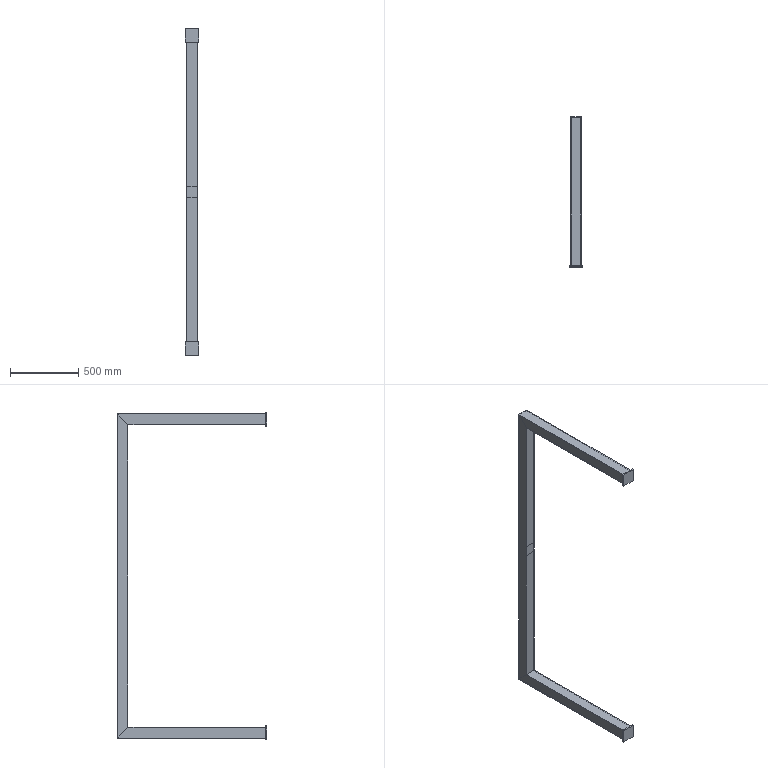Part | STEP file | Outer frame 1 | 2 solids | 42 faces | box 100 x 1100 x 2400 mm | volume 6796800 mm3 | plane 42
STEP:
#1=CARTESIAN_POINT('',(-50.,0.,-2250.));
#2=VERTEX_POINT('',#1);
#3=CARTESIAN_POINT('',(-50.,0.,-2350.));
#4=VERTEX_POINT('',#3);
#5=CARTESIAN_POINT('',(-50.,0.,-2350.));
#6=DIRECTION('',(0.,0.,-1.));
#7=VECTOR('',#6,1000.);
#8=LINE('',#5,#7);
#9=EDGE_CURVE('',#2,#4,#8,.T.);
#10=ORIENTED_EDGE('',*,*,#9,.T.);
#11=CARTESIAN_POINT('',(-50.,-10.,-2350.));
#12=VERTEX_POINT('',#11);
#13=CARTESIAN_POINT('',(-50.,-10.,-2350.));
#14=DIRECTION('',(0.,1.,0.));
#15=VECTOR('',#14,1000.);
#16=LINE('',#13,#15);
#17=EDGE_CURVE('',#12,#4,#16,.T.);
#18=ORIENTED_EDGE('',*,*,#17,.F.);
#19=CARTESIAN_POINT('',(-50.,-10.,-2250.));
#20=VERTEX_POINT('',#19);
#21=CARTESIAN_POINT('',(-50.,-10.,-2350.));
#22=DIRECTION('',(0.,0.,-1.));
#23=VECTOR('',#22,1000.);
#24=LINE('',#21,#23);
#25=EDGE_CURVE('',#20,#12,#24,.T.);
#26=ORIENTED_EDGE('',*,*,#25,.F.);
#27=CARTESIAN_POINT('',(-50.,-10.,-2250.));
#28=DIRECTION('',(0.,1.,0.));
#29=VECTOR('',#28,1000.);
#30=LINE('',#27,#29);
#31=EDGE_CURVE('',#20,#2,#30,.T.);
#32=ORIENTED_EDGE('',*,*,#31,.T.);
#33=EDGE_LOOP('',(#10,#18,#26,#32));
#34=FACE_OUTER_BOUND('',#33,.T.);
#35=CARTESIAN_POINT('',(-50.,-10.,-2350.));
#36=DIRECTION('',(1.,0.,0.));
#37=DIRECTION('',(0.,0.,-1.));
#38=AXIS2_PLACEMENT_3D('',#35,#36,#37);
#39=PLANE('',#38);
#40=ADVANCED_FACE('',(#34),#39,.F.);
#41=CARTESIAN_POINT('',(50.,0.,-2350.));
#42=VERTEX_POINT('',#41);
#43=CARTESIAN_POINT('',(50.,0.,-2350.));
#44=DIRECTION('',(1.,0.,0.));
#45=VECTOR('',#44,1000.);
#46=LINE('',#43,#45);
#47=EDGE_CURVE('',#4,#42,#46,.T.);
#48=ORIENTED_EDGE('',*,*,#47,.T.);
#49=CARTESIAN_POINT('',(50.,-10.,-2350.));
#50=VERTEX_POINT('',#49);
#51=CARTESIAN_POINT('',(50.,-10.,-2350.));
#52=DIRECTION('',(0.,1.,0.));
#53=VECTOR('',#52,1000.);
#54=LINE('',#51,#53);
#55=EDGE_CURVE('',#50,#42,#54,.T.);
#56=ORIENTED_EDGE('',*,*,#55,.F.);
#57=CARTESIAN_POINT('',(50.,-10.,-2350.));
#58=DIRECTION('',(1.,0.,0.));
#59=VECTOR('',#58,1000.);
#60=LINE('',#57,#59);
#61=EDGE_CURVE('',#12,#50,#60,.T.);
#62=ORIENTED_EDGE('',*,*,#61,.F.);
#63=ORIENTED_EDGE('',*,*,#17,.T.);
#64=EDGE_LOOP('',(#48,#56,#62,#63));
#65=FACE_OUTER_BOUND('',#64,.T.);
#66=CARTESIAN_POINT('',(50.,-10.,-2350.));
#67=DIRECTION('',(0.,0.,1.));
#68=DIRECTION('',(0.,-1.,0.));
#69=AXIS2_PLACEMENT_3D('',#66,#67,#68);
#70=PLANE('',#69);
#71=ADVANCED_FACE('',(#65),#70,.F.);
#72=CARTESIAN_POINT('',(50.,0.,-2250.));
#73=VERTEX_POINT('',#72);
#74=CARTESIAN_POINT('',(50.,0.,-2350.));
#75=DIRECTION('',(0.,0.,1.));
#76=VECTOR('',#75,1000.);
#77=LINE('',#74,#76);
#78=EDGE_CURVE('',#42,#73,#77,.T.);
#79=ORIENTED_EDGE('',*,*,#78,.T.);
#80=CARTESIAN_POINT('',(50.,-10.,-2250.));
#81=VERTEX_POINT('',#80);
#82=CARTESIAN_POINT('',(50.,-10.,-2250.));
#83=DIRECTION('',(0.,1.,0.));
#84=VECTOR('',#83,1000.);
#85=LINE('',#82,#84);
#86=EDGE_CURVE('',#81,#73,#85,.T.);
#87=ORIENTED_EDGE('',*,*,#86,.F.);
#88=CARTESIAN_POINT('',(50.,-10.,-2350.));
#89=DIRECTION('',(0.,0.,1.));
#90=VECTOR('',#89,1000.);
#91=LINE('',#88,#90);
#92=EDGE_CURVE('',#50,#81,#91,.T.);
#93=ORIENTED_EDGE('',*,*,#92,.F.);
#94=ORIENTED_EDGE('',*,*,#55,.T.);
#95=EDGE_LOOP('',(#79,#87,#93,#94));
#96=FACE_OUTER_BOUND('',#95,.T.);
#97=CARTESIAN_POINT('',(50.,-10.,-2350.));
#98=DIRECTION('',(-1.,0.,0.));
#99=DIRECTION('',(0.,0.,1.));
#100=AXIS2_PLACEMENT_3D('',#97,#98,#99);
#101=PLANE('',#100);
#102=ADVANCED_FACE('',(#96),#101,.F.);
#103=CARTESIAN_POINT('',(50.,0.,-2250.));
#104=DIRECTION('',(-1.,0.,0.));
#105=VECTOR('',#104,1000.);
#106=LINE('',#103,#105);
#107=EDGE_CURVE('',#73,#2,#106,.T.);
#108=ORIENTED_EDGE('',*,*,#107,.T.);
#109=ORIENTED_EDGE('',*,*,#31,.F.);
#110=CARTESIAN_POINT('',(50.,-10.,-2250.));
#111=DIRECTION('',(-1.,0.,0.));
#112=VECTOR('',#111,1000.);
#113=LINE('',#110,#112);
#114=EDGE_CURVE('',#81,#20,#113,.T.);
#115=ORIENTED_EDGE('',*,*,#114,.F.);
#116=ORIENTED_EDGE('',*,*,#86,.T.);
#117=EDGE_LOOP('',(#108,#109,#115,#116));
#118=FACE_OUTER_BOUND('',#117,.T.);
#119=CARTESIAN_POINT('',(50.,-10.,-2250.));
#120=DIRECTION('',(0.,0.,-1.));
#121=DIRECTION('',(0.,1.,0.));
#122=AXIS2_PLACEMENT_3D('',#119,#120,#121);
#123=PLANE('',#122);
#124=ADVANCED_FACE('',(#118),#123,.F.);
#125=ORIENTED_EDGE('',*,*,#25,.T.);
#126=ORIENTED_EDGE('',*,*,#61,.T.);
#127=ORIENTED_EDGE('',*,*,#92,.T.);
#128=ORIENTED_EDGE('',*,*,#114,.T.);
#129=EDGE_LOOP('',(#125,#126,#127,#128));
#130=FACE_OUTER_BOUND('',#129,.T.);
#131=CARTESIAN_POINT('',(0.,-10.,0.));
#132=DIRECTION('',(0.,-1.,0.));
#133=DIRECTION('',(0.,0.,-1.));
#134=AXIS2_PLACEMENT_3D('',#131,#132,#133);
#135=PLANE('',#134);
#136=ADVANCED_FACE('',(#130),#135,.T.);
#137=ORIENTED_EDGE('',*,*,#9,.F.);
#138=ORIENTED_EDGE('',*,*,#107,.F.);
#139=ORIENTED_EDGE('',*,*,#78,.F.);
#140=ORIENTED_EDGE('',*,*,#47,.F.);
#141=EDGE_LOOP('',(#137,#138,#139,#140));
#142=FACE_OUTER_BOUND('',#141,.T.);
#143=CARTESIAN_POINT('',(0.,0.,0.));
#144=DIRECTION('',(0.,-1.,0.));
#145=DIRECTION('',(0.,0.,-1.));
#146=AXIS2_PLACEMENT_3D('',#143,#144,#145);
#147=PLANE('',#146);
#148=ADVANCED_FACE('',(#142),#147,.F.);
#149=CLOSED_SHELL('',(#40,#71,#102,#124,#136,#148));
#150=MANIFOLD_SOLID_BREP('',#149);
#151=CARTESIAN_POINT('',(40.,1010.,-1190.5));
#152=VERTEX_POINT('',#151);
#153=CARTESIAN_POINT('',(40.,1010.,-2260.));
#154=VERTEX_POINT('',#153);
#155=CARTESIAN_POINT('',(40.,1010.,44.1));
#156=DIRECTION('',(0.,0.,-1.));
#157=VECTOR('',#156,1000.);
#158=LINE('',#155,#157);
#159=EDGE_CURVE('',#152,#154,#158,.T.);
#160=ORIENTED_EDGE('',*,*,#159,.F.);
#161=CARTESIAN_POINT('',(-40.,1010.,-1190.5));
#162=VERTEX_POINT('',#161);
#163=CARTESIAN_POINT('',(40.,1010.,-1190.5));
#164=DIRECTION('',(1.,0.,0.));
#165=VECTOR('',#164,1000.);
#166=LINE('',#163,#165);
#167=EDGE_CURVE('',#162,#152,#166,.T.);
#168=ORIENTED_EDGE('',*,*,#167,.F.);
#169=CARTESIAN_POINT('',(-40.,1010.,-2260.));
#170=VERTEX_POINT('',#169);
#171=CARTESIAN_POINT('',(-40.,1010.,44.1));
#172=DIRECTION('',(0.,0.,-1.));
#173=VECTOR('',#172,1000.);
#174=LINE('',#171,#173);
#175=EDGE_CURVE('',#162,#170,#174,.T.);
#176=ORIENTED_EDGE('',*,*,#175,.T.);
#177=CARTESIAN_POINT('',(40.,1010.,-2260.));
#178=DIRECTION('',(1.,0.,0.));
#179=VECTOR('',#178,1000.);
#180=LINE('',#177,#179);
#181=EDGE_CURVE('',#170,#154,#180,.T.);
#182=ORIENTED_EDGE('',*,*,#181,.T.);
#183=EDGE_LOOP('',(#160,#168,#176,#182));
#184=FACE_OUTER_BOUND('',#183,.T.);
#185=CARTESIAN_POINT('',(40.,1010.,44.1));
#186=DIRECTION('',(0.,-1.,0.));
#187=DIRECTION('',(1.,0.,0.));
#188=AXIS2_PLACEMENT_3D('',#185,#186,#187);
#189=PLANE('',#188);
#190=ADVANCED_FACE('',(#184),#189,.T.);
#191=CARTESIAN_POINT('',(-40.,1010.,-40.));
#192=VERTEX_POINT('',#191);
#193=CARTESIAN_POINT('',(-40.,1010.,-1110.5));
#194=VERTEX_POINT('',#193);
#195=CARTESIAN_POINT('',(-40.,1010.,44.1));
#196=DIRECTION('',(0.,0.,-1.));
#197=VECTOR('',#196,1000.);
#198=LINE('',#195,#197);
#199=EDGE_CURVE('',#192,#194,#198,.T.);
#200=ORIENTED_EDGE('',*,*,#199,.T.);
#201=CARTESIAN_POINT('',(40.,1010.,-1110.5));
#202=VERTEX_POINT('',#201);
#203=CARTESIAN_POINT('',(40.,1010.,-1110.5));
#204=DIRECTION('',(-1.,0.,0.));
#205=VECTOR('',#204,1000.);
#206=LINE('',#203,#205);
#207=EDGE_CURVE('',#202,#194,#206,.T.);
#208=ORIENTED_EDGE('',*,*,#207,.F.);
#209=CARTESIAN_POINT('',(40.,1010.,-40.));
#210=VERTEX_POINT('',#209);
#211=CARTESIAN_POINT('',(40.,1010.,44.1));
#212=DIRECTION('',(0.,0.,-1.));
#213=VECTOR('',#212,1000.);
#214=LINE('',#211,#213);
#215=EDGE_CURVE('',#210,#202,#214,.T.);
#216=ORIENTED_EDGE('',*,*,#215,.F.);
#217=CARTESIAN_POINT('',(40.,1010.,-40.));
#218=DIRECTION('',(1.,0.,0.));
#219=VECTOR('',#218,1000.);
#220=LINE('',#217,#219);
#221=EDGE_CURVE('',#192,#210,#220,.T.);
#222=ORIENTED_EDGE('',*,*,#221,.F.);
#223=EDGE_LOOP('',(#200,#208,#216,#222));
#224=FACE_OUTER_BOUND('',#223,.T.);
#225=CARTESIAN_POINT('',(40.,1010.,44.1));
#226=DIRECTION('',(0.,-1.,0.));
#227=DIRECTION('',(1.,0.,0.));
#228=AXIS2_PLACEMENT_3D('',#225,#226,#227);
#229=PLANE('',#228);
#230=ADVANCED_FACE('',(#224),#229,.T.);
#231=CARTESIAN_POINT('',(35.,0.,-35.));
#232=VERTEX_POINT('',#231);
#233=CARTESIAN_POINT('',(35.,1015.,-35.));
#234=VERTEX_POINT('',#233);
#235=CARTESIAN_POINT('',(35.,0.,-35.));
#236=DIRECTION('',(0.,1.,0.));
#237=VECTOR('',#236,1000.);
#238=LINE('',#235,#237);
#239=EDGE_CURVE('',#232,#234,#238,.T.);
#240=ORIENTED_EDGE('',*,*,#239,.T.);
#241=CARTESIAN_POINT('',(-35.,1015.,-35.));
#242=VERTEX_POINT('',#241);
#243=CARTESIAN_POINT('',(35.,1015.,-35.));
#244=DIRECTION('',(-1.,0.,0.));
#245=VECTOR('',#244,1000.);
#246=LINE('',#243,#245);
#247=EDGE_CURVE('',#234,#242,#246,.T.);
#248=ORIENTED_EDGE('',*,*,#247,.T.);
#249=CARTESIAN_POINT('',(-35.,0.,-35.));
#250=VERTEX_POINT('',#249);
#251=CARTESIAN_POINT('',(-35.,0.,-35.));
#252=DIRECTION('',(0.,1.,0.));
#253=VECTOR('',#252,1000.);
#254=LINE('',#251,#253);
#255=EDGE_CURVE('',#250,#242,#254,.T.);
#256=ORIENTED_EDGE('',*,*,#255,.F.);
#257=CARTESIAN_POINT('',(35.,0.,-35.));
#258=DIRECTION('',(1.,0.,0.));
#259=VECTOR('',#258,1000.);
#260=LINE('',#257,#259);
#261=EDGE_CURVE('',#250,#232,#260,.T.);
#262=ORIENTED_EDGE('',*,*,#261,.T.);
#263=EDGE_LOOP('',(#240,#248,#256,#262));
#264=FACE_OUTER_BOUND('',#263,.T.);
#265=CARTESIAN_POINT('',(35.,0.,-35.));
#266=DIRECTION('',(0.,0.,1.));
#267=DIRECTION('',(1.,0.,0.));
#268=AXIS2_PLACEMENT_3D('',#265,#266,#267);
#269=PLANE('',#268);
#270=ADVANCED_FACE('',(#264),#269,.T.);
#271=CARTESIAN_POINT('',(35.,0.,35.));
#272=VERTEX_POINT('',#271);
#273=CARTESIAN_POINT('',(35.,1085.,35.));
#274=VERTEX_POINT('',#273);
#275=CARTESIAN_POINT('',(35.,0.,35.));
#276=DIRECTION('',(0.,1.,0.));
#277=VECTOR('',#276,1000.);
#278=LINE('',#275,#277);
#279=EDGE_CURVE('',#272,#274,#278,.T.);
#280=ORIENTED_EDGE('',*,*,#279,.T.);
#281=CARTESIAN_POINT('',(35.,542.5,-507.5));
#282=DIRECTION('',(0.,-0.7071,-0.7071));
#283=VECTOR('',#282,1000.);
#284=LINE('',#281,#283);
#285=EDGE_CURVE('',#274,#234,#284,.T.);
#286=ORIENTED_EDGE('',*,*,#285,.T.);
#287=ORIENTED_EDGE('',*,*,#239,.F.);
#288=CARTESIAN_POINT('',(35.,0.,35.));
#289=DIRECTION('',(0.,0.,1.));
#290=VECTOR('',#289,1000.);
#291=LINE('',#288,#290);
#292=EDGE_CURVE('',#232,#272,#291,.T.);
#293=ORIENTED_EDGE('',*,*,#292,.T.);
#294=EDGE_LOOP('',(#280,#286,#287,#293));
#295=FACE_OUTER_BOUND('',#294,.T.);
#296=CARTESIAN_POINT('',(35.,0.,35.));
#297=DIRECTION('',(-1.,0.,0.));
#298=DIRECTION('',(0.,0.,1.));
#299=AXIS2_PLACEMENT_3D('',#296,#297,#298);
#300=PLANE('',#299);
#301=ADVANCED_FACE('',(#295),#300,.T.);
#302=CARTESIAN_POINT('',(-35.,0.,35.));
#303=VERTEX_POINT('',#302);
#304=CARTESIAN_POINT('',(-35.,1085.,35.));
#305=VERTEX_POINT('',#304);
#306=CARTESIAN_POINT('',(-35.,0.,35.));
#307=DIRECTION('',(0.,1.,0.));
#308=VECTOR('',#307,1000.);
#309=LINE('',#306,#308);
#310=EDGE_CURVE('',#303,#305,#309,.T.);
#311=ORIENTED_EDGE('',*,*,#310,.T.);
#312=CARTESIAN_POINT('',(35.,1085.,35.));
#313=DIRECTION('',(1.,0.,0.));
#314=VECTOR('',#313,1000.);
#315=LINE('',#312,#314);
#316=EDGE_CURVE('',#305,#274,#315,.T.);
#317=ORIENTED_EDGE('',*,*,#316,.T.);
#318=ORIENTED_EDGE('',*,*,#279,.F.);
#319=CARTESIAN_POINT('',(35.,0.,35.));
#320=DIRECTION('',(-1.,0.,0.));
#321=VECTOR('',#320,1000.);
#322=LINE('',#319,#321);
#323=EDGE_CURVE('',#272,#303,#322,.T.);
#324=ORIENTED_EDGE('',*,*,#323,.T.);
#325=EDGE_LOOP('',(#311,#317,#318,#324));
#326=FACE_OUTER_BOUND('',#325,.T.);
#327=CARTESIAN_POINT('',(35.,0.,35.));
#328=DIRECTION('',(0.,0.,-1.));
#329=DIRECTION('',(0.,1.,0.));
#330=AXIS2_PLACEMENT_3D('',#327,#328,#329);
#331=PLANE('',#330);
#332=ADVANCED_FACE('',(#326),#331,.T.);
#333=ORIENTED_EDGE('',*,*,#255,.T.);
#334=CARTESIAN_POINT('',(-35.,542.5,-507.5));
#335=DIRECTION('',(0.,0.7071,0.7071));
#336=VECTOR('',#335,1000.);
#337=LINE('',#334,#336);
#338=EDGE_CURVE('',#242,#305,#337,.T.);
#339=ORIENTED_EDGE('',*,*,#338,.T.);
#340=ORIENTED_EDGE('',*,*,#310,.F.);
#341=CARTESIAN_POINT('',(-35.,0.,35.));
#342=DIRECTION('',(0.,0.,-1.));
#343=VECTOR('',#342,1000.);
#344=LINE('',#341,#343);
#345=EDGE_CURVE('',#303,#250,#344,.T.);
#346=ORIENTED_EDGE('',*,*,#345,.T.);
#347=EDGE_LOOP('',(#333,#339,#340,#346));
#348=FACE_OUTER_BOUND('',#347,.T.);
#349=CARTESIAN_POINT('',(-35.,0.,35.));
#350=DIRECTION('',(1.,0.,0.));
#351=DIRECTION('',(0.,0.,-1.));
#352=AXIS2_PLACEMENT_3D('',#349,#350,#351);
#353=PLANE('',#352);
#354=ADVANCED_FACE('',(#348),#353,.T.);
#355=CARTESIAN_POINT('',(35.,1015.,-2265.));
#356=VERTEX_POINT('',#355);
#357=CARTESIAN_POINT('',(35.,1015.,38.6));
#358=DIRECTION('',(0.,0.,-1.));
#359=VECTOR('',#358,1000.);
#360=LINE('',#357,#359);
#361=EDGE_CURVE('',#234,#356,#360,.T.);
#362=ORIENTED_EDGE('',*,*,#361,.T.);
#363=CARTESIAN_POINT('',(-35.,1015.,-2265.));
#364=VERTEX_POINT('',#363);
#365=CARTESIAN_POINT('',(35.,1015.,-2265.));
#366=DIRECTION('',(-1.,0.,0.));
#367=VECTOR('',#366,1000.);
#368=LINE('',#365,#367);
#369=EDGE_CURVE('',#356,#364,#368,.T.);
#370=ORIENTED_EDGE('',*,*,#369,.T.);
#371=CARTESIAN_POINT('',(-35.,1015.,38.6));
#372=DIRECTION('',(0.,0.,-1.));
#373=VECTOR('',#372,1000.);
#374=LINE('',#371,#373);
#375=EDGE_CURVE('',#242,#364,#374,.T.);
#376=ORIENTED_EDGE('',*,*,#375,.F.);
#377=ORIENTED_EDGE('',*,*,#247,.F.);
#378=EDGE_LOOP('',(#362,#370,#376,#377));
#379=FACE_OUTER_BOUND('',#378,.T.);
#380=CARTESIAN_POINT('',(35.,1015.,38.6));
#381=DIRECTION('',(0.,1.,0.));
#382=DIRECTION('',(-1.,0.,0.));
#383=AXIS2_PLACEMENT_3D('',#380,#381,#382);
#384=PLANE('',#383);
#385=ADVANCED_FACE('',(#379),#384,.T.);
#386=CARTESIAN_POINT('',(35.,1085.,-2335.));
#387=VERTEX_POINT('',#386);
#388=CARTESIAN_POINT('',(35.,1085.,38.6));
#389=DIRECTION('',(0.,0.,-1.));
#390=VECTOR('',#389,1000.);
#391=LINE('',#388,#390);
#392=EDGE_CURVE('',#274,#387,#391,.T.);
#393=ORIENTED_EDGE('',*,*,#392,.T.);
#394=CARTESIAN_POINT('',(35.,-101.8,-1148.2));
#395=DIRECTION('',(0.,-0.7071,0.7071));
#396=VECTOR('',#395,1000.);
#397=LINE('',#394,#396);
#398=EDGE_CURVE('',#387,#356,#397,.T.);
#399=ORIENTED_EDGE('',*,*,#398,.T.);
#400=ORIENTED_EDGE('',*,*,#361,.F.);
#401=ORIENTED_EDGE('',*,*,#285,.F.);
#402=EDGE_LOOP('',(#393,#399,#400,#401));
#403=FACE_OUTER_BOUND('',#402,.T.);
#404=CARTESIAN_POINT('',(35.,1085.,38.6));
#405=DIRECTION('',(-1.,0.,0.));
#406=DIRECTION('',(0.,0.,1.));
#407=AXIS2_PLACEMENT_3D('',#404,#405,#406);
#408=PLANE('',#407);
#409=ADVANCED_FACE('',(#403),#408,.T.);
#410=CARTESIAN_POINT('',(-35.,1085.,-2335.));
#411=VERTEX_POINT('',#410);
#412=CARTESIAN_POINT('',(-35.,1085.,38.6));
#413=DIRECTION('',(0.,0.,-1.));
#414=VECTOR('',#413,1000.);
#415=LINE('',#412,#414);
#416=EDGE_CURVE('',#305,#411,#415,.T.);
#417=ORIENTED_EDGE('',*,*,#416,.T.);
#418=CARTESIAN_POINT('',(35.,1085.,-2335.));
#419=DIRECTION('',(1.,0.,0.));
#420=VECTOR('',#419,1000.);
#421=LINE('',#418,#420);
#422=EDGE_CURVE('',#411,#387,#421,.T.);
#423=ORIENTED_EDGE('',*,*,#422,.T.);
#424=ORIENTED_EDGE('',*,*,#392,.F.);
#425=ORIENTED_EDGE('',*,*,#316,.F.);
#426=EDGE_LOOP('',(#417,#423,#424,#425));
#427=FACE_OUTER_BOUND('',#426,.T.);
#428=CARTESIAN_POINT('',(35.,1085.,38.6));
#429=DIRECTION('',(0.,-1.,0.));
#430=DIRECTION('',(0.,0.,-1.));
#431=AXIS2_PLACEMENT_3D('',#428,#429,#430);
#432=PLANE('',#431);
#433=ADVANCED_FACE('',(#427),#432,.T.);
#434=ORIENTED_EDGE('',*,*,#375,.T.);
#435=CARTESIAN_POINT('',(-35.,-101.8,-1148.2));
#436=DIRECTION('',(0.,0.7071,-0.7071));
#437=VECTOR('',#436,1000.);
#438=LINE('',#435,#437);
#439=EDGE_CURVE('',#364,#411,#438,.T.);
#440=ORIENTED_EDGE('',*,*,#439,.T.);
#441=ORIENTED_EDGE('',*,*,#416,.F.);
#442=ORIENTED_EDGE('',*,*,#338,.F.);
#443=EDGE_LOOP('',(#434,#440,#441,#442));
#444=FACE_OUTER_BOUND('',#443,.T.);
#445=CARTESIAN_POINT('',(-35.,1085.,38.6));
#446=DIRECTION('',(1.,0.,0.));
#447=DIRECTION('',(0.,0.,-1.));
#448=AXIS2_PLACEMENT_3D('',#445,#446,#447);
#449=PLANE('',#448);
#450=ADVANCED_FACE('',(#444),#449,.T.);
#451=ORIENTED_EDGE('',*,*,#439,.F.);
#452=CARTESIAN_POINT('',(-35.,0.,-2265.));
#453=VERTEX_POINT('',#452);
#454=CARTESIAN_POINT('',(-35.,1088.6,-2265.));
#455=DIRECTION('',(0.,-1.,0.));
#456=VECTOR('',#455,1000.);
#457=LINE('',#454,#456);
#458=EDGE_CURVE('',#364,#453,#457,.T.);
#459=ORIENTED_EDGE('',*,*,#458,.T.);
#460=CARTESIAN_POINT('',(-35.,0.,-2335.));
#461=VERTEX_POINT('',#460);
#462=CARTESIAN_POINT('',(-35.,0.,-2335.));
#463=DIRECTION('',(0.,0.,1.));
#464=VECTOR('',#463,1000.);
#465=LINE('',#462,#464);
#466=EDGE_CURVE('',#461,#453,#465,.T.);
#467=ORIENTED_EDGE('',*,*,#466,.F.);
#468=CARTESIAN_POINT('',(-35.,1088.6,-2335.));
#469=DIRECTION('',(0.,-1.,0.));
#470=VECTOR('',#469,1000.);
#471=LINE('',#468,#470);
#472=EDGE_CURVE('',#411,#461,#471,.T.);
#473=ORIENTED_EDGE('',*,*,#472,.F.);
#474=EDGE_LOOP('',(#451,#459,#467,#473));
#475=FACE_OUTER_BOUND('',#474,.T.);
#476=CARTESIAN_POINT('',(-35.,1088.6,-2335.));
#477=DIRECTION('',(1.,0.,0.));
#478=DIRECTION('',(0.,0.,-1.));
#479=AXIS2_PLACEMENT_3D('',#476,#477,#478);
#480=PLANE('',#479);
#481=ADVANCED_FACE('',(#475),#480,.T.);
#482=ORIENTED_EDGE('',*,*,#422,.F.);
#483=ORIENTED_EDGE('',*,*,#472,.T.);
#484=CARTESIAN_POINT('',(35.,0.,-2335.));
#485=VERTEX_POINT('',#484);
#486=CARTESIAN_POINT('',(35.,0.,-2335.));
#487=DIRECTION('',(-1.,0.,0.));
#488=VECTOR('',#487,1000.);
#489=LINE('',#486,#488);
#490=EDGE_CURVE('',#485,#461,#489,.T.);
#491=ORIENTED_EDGE('',*,*,#490,.F.);
#492=CARTESIAN_POINT('',(35.,1088.6,-2335.));
#493=DIRECTION('',(0.,-1.,0.));
#494=VECTOR('',#493,1000.);
#495=LINE('',#492,#494);
#496=EDGE_CURVE('',#387,#485,#495,.T.);
#497=ORIENTED_EDGE('',*,*,#496,.F.);
#498=EDGE_LOOP('',(#482,#483,#491,#497));
#499=FACE_OUTER_BOUND('',#498,.T.);
#500=CARTESIAN_POINT('',(35.,1088.6,-2335.));
#501=DIRECTION('',(0.,0.,1.));
#502=DIRECTION('',(1.,0.,0.));
#503=AXIS2_PLACEMENT_3D('',#500,#501,#502);
#504=PLANE('',#503);
#505=ADVANCED_FACE('',(#499),#504,.T.);
#506=ORIENTED_EDGE('',*,*,#398,.F.);
#507=ORIENTED_EDGE('',*,*,#496,.T.);
#508=CARTESIAN_POINT('',(35.,0.,-2265.));
#509=VERTEX_POINT('',#508);
#510=CARTESIAN_POINT('',(35.,0.,-2335.));
#511=DIRECTION('',(0.,0.,-1.));
#512=VECTOR('',#511,1000.);
#513=LINE('',#510,#512);
#514=EDGE_CURVE('',#509,#485,#513,.T.);
#515=ORIENTED_EDGE('',*,*,#514,.F.);
#516=CARTESIAN_POINT('',(35.,1088.6,-2265.));
#517=DIRECTION('',(0.,-1.,0.));
#518=VECTOR('',#517,1000.);
#519=LINE('',#516,#518);
#520=EDGE_CURVE('',#356,#509,#519,.T.);
#521=ORIENTED_EDGE('',*,*,#520,.F.);
#522=EDGE_LOOP('',(#506,#507,#515,#521));
#523=FACE_OUTER_BOUND('',#522,.T.);
#524=CARTESIAN_POINT('',(35.,1088.6,-2335.));
#525=DIRECTION('',(-1.,0.,0.));
#526=DIRECTION('',(0.,0.,1.));
#527=AXIS2_PLACEMENT_3D('',#524,#525,#526);
#528=PLANE('',#527);
#529=ADVANCED_FACE('',(#523),#528,.T.);
#530=ORIENTED_EDGE('',*,*,#369,.F.);
#531=ORIENTED_EDGE('',*,*,#520,.T.);
#532=CARTESIAN_POINT('',(35.,0.,-2265.));
#533=DIRECTION('',(1.,0.,0.));
#534=VECTOR('',#533,1000.);
#535=LINE('',#532,#534);
#536=EDGE_CURVE('',#453,#509,#535,.T.);
#537=ORIENTED_EDGE('',*,*,#536,.F.);
#538=ORIENTED_EDGE('',*,*,#458,.F.);
#539=EDGE_LOOP('',(#530,#531,#537,#538));
#540=FACE_OUTER_BOUND('',#539,.T.);
#541=CARTESIAN_POINT('',(35.,1088.6,-2265.));
#542=DIRECTION('',(0.,0.,-1.));
#543=DIRECTION('',(-1.,0.,0.));
#544=AXIS2_PLACEMENT_3D('',#541,#542,#543);
#545=PLANE('',#544);
#546=ADVANCED_FACE('',(#540),#545,.T.);
#547=ORIENTED_EDGE('',*,*,#466,.T.);
#548=ORIENTED_EDGE('',*,*,#536,.T.);
#549=ORIENTED_EDGE('',*,*,#514,.T.);
#550=ORIENTED_EDGE('',*,*,#490,.T.);
#551=EDGE_LOOP('',(#547,#548,#549,#550));
#552=FACE_BOUND('',#551,.T.);
#553=CARTESIAN_POINT('',(-40.,0.,-2260.));
#554=VERTEX_POINT('',#553);
#555=CARTESIAN_POINT('',(-40.,0.,-2340.));
#556=VERTEX_POINT('',#555);
#557=CARTESIAN_POINT('',(-40.,0.,-2340.));
#558=DIRECTION('',(0.,0.,-1.));
#559=VECTOR('',#558,1000.);
#560=LINE('',#557,#559);
#561=EDGE_CURVE('',#554,#556,#560,.T.);
#562=ORIENTED_EDGE('',*,*,#561,.T.);
#563=CARTESIAN_POINT('',(40.,0.,-2340.));
#564=VERTEX_POINT('',#563);
#565=CARTESIAN_POINT('',(40.,0.,-2340.));
#566=DIRECTION('',(1.,0.,0.));
#567=VECTOR('',#566,1000.);
#568=LINE('',#565,#567);
#569=EDGE_CURVE('',#556,#564,#568,.T.);
#570=ORIENTED_EDGE('',*,*,#569,.T.);
#571=CARTESIAN_POINT('',(40.,0.,-2260.));
#572=VERTEX_POINT('',#571);
#573=CARTESIAN_POINT('',(40.,0.,-2340.));
#574=DIRECTION('',(0.,0.,1.));
#575=VECTOR('',#574,1000.);
#576=LINE('',#573,#575);
#577=EDGE_CURVE('',#564,#572,#576,.T.);
#578=ORIENTED_EDGE('',*,*,#577,.T.);
#579=CARTESIAN_POINT('',(40.,0.,-2260.));
#580=DIRECTION('',(-1.,0.,0.));
#581=VECTOR('',#580,1000.);
#582=LINE('',#579,#581);
#583=EDGE_CURVE('',#572,#554,#582,.T.);
#584=ORIENTED_EDGE('',*,*,#583,.T.);
#585=EDGE_LOOP('',(#562,#570,#578,#584));
#586=FACE_OUTER_BOUND('',#585,.T.);
#587=CARTESIAN_POINT('',(0.,0.,-2300.));
#588=DIRECTION('',(0.,-1.,0.));
#589=DIRECTION('',(0.,0.,-1.));
#590=AXIS2_PLACEMENT_3D('',#587,#588,#589);
#591=PLANE('',#590);
#592=ADVANCED_FACE('',(#552,#586),#591,.T.);
#593=CARTESIAN_POINT('',(40.,0.,-40.));
#594=VERTEX_POINT('',#593);
#595=CARTESIAN_POINT('',(40.,0.,-40.));
#596=DIRECTION('',(0.,1.,0.));
#597=VECTOR('',#596,1000.);
#598=LINE('',#595,#597);
#599=EDGE_CURVE('',#594,#210,#598,.T.);
#600=ORIENTED_EDGE('',*,*,#599,.T.);
#601=CARTESIAN_POINT('',(40.,1090.,40.));
#602=VERTEX_POINT('',#601);
#603=CARTESIAN_POINT('',(40.,545.,-505.));
#604=DIRECTION('',(0.,0.7071,0.7071));
#605=VECTOR('',#604,1000.);
#606=LINE('',#603,#605);
#607=EDGE_CURVE('',#210,#602,#606,.T.);
#608=ORIENTED_EDGE('',*,*,#607,.T.);
#609=CARTESIAN_POINT('',(40.,0.,40.));
#610=VERTEX_POINT('',#609);
#611=CARTESIAN_POINT('',(40.,0.,40.));
#612=DIRECTION('',(0.,1.,0.));
#613=VECTOR('',#612,1000.);
#614=LINE('',#611,#613);
#615=EDGE_CURVE('',#610,#602,#614,.T.);
#616=ORIENTED_EDGE('',*,*,#615,.F.);
#617=CARTESIAN_POINT('',(40.,0.,40.));
#618=DIRECTION('',(0.,0.,-1.));
#619=VECTOR('',#618,1000.);
#620=LINE('',#617,#619);
#621=EDGE_CURVE('',#610,#594,#620,.T.);
#622=ORIENTED_EDGE('',*,*,#621,.T.);
#623=EDGE_LOOP('',(#600,#608,#616,#622));
#624=FACE_OUTER_BOUND('',#623,.T.);
#625=CARTESIAN_POINT('',(40.,0.,40.));
#626=DIRECTION('',(1.,0.,0.));
#627=DIRECTION('',(0.,0.,-1.));
#628=AXIS2_PLACEMENT_3D('',#625,#626,#627);
#629=PLANE('',#628);
#630=ADVANCED_FACE('',(#624),#629,.T.);
#631=CARTESIAN_POINT('',(-40.,0.,-40.));
#632=VERTEX_POINT('',#631);
#633=CARTESIAN_POINT('',(-40.,0.,-40.));
#634=DIRECTION('',(0.,1.,0.));
#635=VECTOR('',#634,1000.);
#636=LINE('',#633,#635);
#637=EDGE_CURVE('',#632,#192,#636,.T.);
#638=ORIENTED_EDGE('',*,*,#637,.T.);
#639=ORIENTED_EDGE('',*,*,#221,.T.);
#640=ORIENTED_EDGE('',*,*,#599,.F.);
#641=CARTESIAN_POINT('',(40.,0.,-40.));
#642=DIRECTION('',(-1.,0.,0.));
#643=VECTOR('',#642,1000.);
#644=LINE('',#641,#643);
#645=EDGE_CURVE('',#594,#632,#644,.T.);
#646=ORIENTED_EDGE('',*,*,#645,.T.);
#647=EDGE_LOOP('',(#638,#639,#640,#646));
#648=FACE_OUTER_BOUND('',#647,.T.);
#649=CARTESIAN_POINT('',(40.,0.,-40.));
#650=DIRECTION('',(0.,0.,-1.));
#651=DIRECTION('',(-1.,0.,0.));
#652=AXIS2_PLACEMENT_3D('',#649,#650,#651);
#653=PLANE('',#652);
#654=ADVANCED_FACE('',(#648),#653,.T.);
#655=CARTESIAN_POINT('',(-40.,0.,40.));
#656=VERTEX_POINT('',#655);
#657=CARTESIAN_POINT('',(-40.,1090.,40.));
#658=VERTEX_POINT('',#657);
#659=CARTESIAN_POINT('',(-40.,0.,40.));
#660=DIRECTION('',(0.,1.,0.));
#661=VECTOR('',#660,1000.);
#662=LINE('',#659,#661);
#663=EDGE_CURVE('',#656,#658,#662,.T.);
#664=ORIENTED_EDGE('',*,*,#663,.T.);
#665=CARTESIAN_POINT('',(-40.,545.,-505.));
#666=DIRECTION('',(0.,-0.7071,-0.7071));
#667=VECTOR('',#666,1000.);
#668=LINE('',#665,#667);
#669=EDGE_CURVE('',#658,#192,#668,.T.);
#670=ORIENTED_EDGE('',*,*,#669,.T.);
#671=ORIENTED_EDGE('',*,*,#637,.F.);
#672=CARTESIAN_POINT('',(-40.,0.,40.));
#673=DIRECTION('',(0.,0.,1.));
#674=VECTOR('',#673,1000.);
#675=LINE('',#672,#674);
#676=EDGE_CURVE('',#632,#656,#675,.T.);
#677=ORIENTED_EDGE('',*,*,#676,.T.);
#678=EDGE_LOOP('',(#664,#670,#671,#677));
#679=FACE_OUTER_BOUND('',#678,.T.);
#680=CARTESIAN_POINT('',(-40.,0.,40.));
#681=DIRECTION('',(-1.,0.,0.));
#682=DIRECTION('',(0.,0.,1.));
#683=AXIS2_PLACEMENT_3D('',#680,#681,#682);
#684=PLANE('',#683);
#685=ADVANCED_FACE('',(#679),#684,.T.);
#686=ORIENTED_EDGE('',*,*,#615,.T.);
#687=CARTESIAN_POINT('',(40.,1090.,40.));
#688=DIRECTION('',(-1.,0.,0.));
#689=VECTOR('',#688,1000.);
#690=LINE('',#687,#689);
#691=EDGE_CURVE('',#602,#658,#690,.T.);
#692=ORIENTED_EDGE('',*,*,#691,.T.);
#693=ORIENTED_EDGE('',*,*,#663,.F.);
#694=CARTESIAN_POINT('',(40.,0.,40.));
#695=DIRECTION('',(1.,0.,0.));
#696=VECTOR('',#695,1000.);
#697=LINE('',#694,#696);
#698=EDGE_CURVE('',#656,#610,#697,.T.);
#699=ORIENTED_EDGE('',*,*,#698,.T.);
#700=EDGE_LOOP('',(#686,#692,#693,#699));
#701=FACE_OUTER_BOUND('',#700,.T.);
#702=CARTESIAN_POINT('',(40.,0.,40.));
#703=DIRECTION('',(0.,0.,1.));
#704=DIRECTION('',(1.,0.,0.));
#705=AXIS2_PLACEMENT_3D('',#702,#703,#704);
#706=PLANE('',#705);
#707=ADVANCED_FACE('',(#701),#706,.T.);
#708=CARTESIAN_POINT('',(40.,1010.5,-1110.5));
#709=VERTEX_POINT('',#708);
#710=CARTESIAN_POINT('',(40.,1010.5,-1110.5));
#711=DIRECTION('',(0.,-1.,0.));
#712=VECTOR('',#711,1000.);
#713=LINE('',#710,#712);
#714=EDGE_CURVE('',#709,#202,#713,.T.);
#715=ORIENTED_EDGE('',*,*,#714,.F.);
#716=CARTESIAN_POINT('',(40.,1010.5,-1190.5));
#717=VERTEX_POINT('',#716);
#718=CARTESIAN_POINT('',(40.,1010.5,-1110.5));
#719=DIRECTION('',(0.,0.,1.));
#720=VECTOR('',#719,1000.);
#721=LINE('',#718,#720);
#722=EDGE_CURVE('',#717,#709,#721,.T.);
#723=ORIENTED_EDGE('',*,*,#722,.F.);
#724=CARTESIAN_POINT('',(40.,1010.5,-1190.5));
#725=DIRECTION('',(0.,-1.,0.));
#726=VECTOR('',#725,1000.);
#727=LINE('',#724,#726);
#728=EDGE_CURVE('',#717,#152,#727,.T.);
#729=ORIENTED_EDGE('',*,*,#728,.T.);
#730=ORIENTED_EDGE('',*,*,#159,.T.);
#731=CARTESIAN_POINT('',(40.,1090.,-2340.));
#732=VERTEX_POINT('',#731);
#733=CARTESIAN_POINT('',(40.,-102.05,-1147.95));
#734=DIRECTION('',(0.,0.7071,-0.7071));
#735=VECTOR('',#734,1000.);
#736=LINE('',#733,#735);
#737=EDGE_CURVE('',#154,#732,#736,.T.);
#738=ORIENTED_EDGE('',*,*,#737,.T.);
#739=CARTESIAN_POINT('',(40.,1090.,44.1));
#740=DIRECTION('',(0.,0.,-1.));
#741=VECTOR('',#740,1000.);
#742=LINE('',#739,#741);
#743=EDGE_CURVE('',#602,#732,#742,.T.);
#744=ORIENTED_EDGE('',*,*,#743,.F.);
#745=ORIENTED_EDGE('',*,*,#607,.F.);
#746=ORIENTED_EDGE('',*,*,#215,.T.);
#747=EDGE_LOOP('',(#715,#723,#729,#730,#738,#744,#745,#746));
#748=FACE_OUTER_BOUND('',#747,.T.);
#749=CARTESIAN_POINT('',(40.,1090.,44.1));
#750=DIRECTION('',(1.,0.,0.));
#751=DIRECTION('',(0.,0.,-1.));
#752=AXIS2_PLACEMENT_3D('',#749,#750,#751);
#753=PLANE('',#752);
#754=ADVANCED_FACE('',(#748),#753,.T.);
#755=CARTESIAN_POINT('',(-40.,1010.5,-1110.5));
#756=VERTEX_POINT('',#755);
#757=CARTESIAN_POINT('',(-40.,1010.5,-1110.5));
#758=DIRECTION('',(0.,-1.,0.));
#759=VECTOR('',#758,1000.);
#760=LINE('',#757,#759);
#761=EDGE_CURVE('',#756,#194,#760,.T.);
#762=ORIENTED_EDGE('',*,*,#761,.T.);
#763=ORIENTED_EDGE('',*,*,#199,.F.);
#764=ORIENTED_EDGE('',*,*,#669,.F.);
#765=CARTESIAN_POINT('',(-40.,1090.,-2340.));
#766=VERTEX_POINT('',#765);
#767=CARTESIAN_POINT('',(-40.,1090.,44.1));
#768=DIRECTION('',(0.,0.,-1.));
#769=VECTOR('',#768,1000.);
#770=LINE('',#767,#769);
#771=EDGE_CURVE('',#658,#766,#770,.T.);
#772=ORIENTED_EDGE('',*,*,#771,.T.);
#773=CARTESIAN_POINT('',(-40.,-102.05,-1147.95));
#774=DIRECTION('',(0.,-0.7071,0.7071));
#775=VECTOR('',#774,1000.);
#776=LINE('',#773,#775);
#777=EDGE_CURVE('',#766,#170,#776,.T.);
#778=ORIENTED_EDGE('',*,*,#777,.T.);
#779=ORIENTED_EDGE('',*,*,#175,.F.);
#780=CARTESIAN_POINT('',(-40.,1010.5,-1190.5));
#781=VERTEX_POINT('',#780);
#782=CARTESIAN_POINT('',(-40.,1010.5,-1190.5));
#783=DIRECTION('',(0.,-1.,0.));
#784=VECTOR('',#783,1000.);
#785=LINE('',#782,#784);
#786=EDGE_CURVE('',#781,#162,#785,.T.);
#787=ORIENTED_EDGE('',*,*,#786,.F.);
#788=CARTESIAN_POINT('',(-40.,1010.5,-1110.5));
#789=DIRECTION('',(0.,0.,-1.));
#790=VECTOR('',#789,1000.);
#791=LINE('',#788,#790);
#792=EDGE_CURVE('',#756,#781,#791,.T.);
#793=ORIENTED_EDGE('',*,*,#792,.F.);
#794=EDGE_LOOP('',(#762,#763,#764,#772,#778,#779,#787,#793));
#795=FACE_OUTER_BOUND('',#794,.T.);
#796=CARTESIAN_POINT('',(-40.,1090.,44.1));
#797=DIRECTION('',(-1.,0.,0.));
#798=DIRECTION('',(0.,0.,1.));
#799=AXIS2_PLACEMENT_3D('',#796,#797,#798);
#800=PLANE('',#799);
#801=ADVANCED_FACE('',(#795),#800,.T.);
#802=ORIENTED_EDGE('',*,*,#743,.T.);
#803=CARTESIAN_POINT('',(40.,1090.,-2340.));
#804=DIRECTION('',(-1.,0.,0.));
#805=VECTOR('',#804,1000.);
#806=LINE('',#803,#805);
#807=EDGE_CURVE('',#732,#766,#806,.T.);
#808=ORIENTED_EDGE('',*,*,#807,.T.);
#809=ORIENTED_EDGE('',*,*,#771,.F.);
#810=ORIENTED_EDGE('',*,*,#691,.F.);
#811=EDGE_LOOP('',(#802,#808,#809,#810));
#812=FACE_OUTER_BOUND('',#811,.T.);
#813=CARTESIAN_POINT('',(40.,1090.,44.1));
#814=DIRECTION('',(0.,1.,0.));
#815=DIRECTION('',(-1.,0.,0.));
#816=AXIS2_PLACEMENT_3D('',#813,#814,#815);
#817=PLANE('',#816);
#818=ADVANCED_FACE('',(#812),#817,.T.);
#819=ORIENTED_EDGE('',*,*,#807,.F.);
#820=CARTESIAN_POINT('',(40.,1094.1,-2340.));
#821=DIRECTION('',(0.,-1.,0.));
#822=VECTOR('',#821,1000.);
#823=LINE('',#820,#822);
#824=EDGE_CURVE('',#732,#564,#823,.T.);
#825=ORIENTED_EDGE('',*,*,#824,.T.);
#826=ORIENTED_EDGE('',*,*,#569,.F.);
#827=CARTESIAN_POINT('',(-40.,1094.1,-2340.));
#828=DIRECTION('',(0.,-1.,0.));
#829=VECTOR('',#828,1000.);
#830=LINE('',#827,#829);
#831=EDGE_CURVE('',#766,#556,#830,.T.);
#832=ORIENTED_EDGE('',*,*,#831,.F.);
#833=EDGE_LOOP('',(#819,#825,#826,#832));
#834=FACE_OUTER_BOUND('',#833,.T.);
#835=CARTESIAN_POINT('',(40.,1094.1,-2340.));
#836=DIRECTION('',(0.,0.,-1.));
#837=DIRECTION('',(-1.,0.,0.));
#838=AXIS2_PLACEMENT_3D('',#835,#836,#837);
#839=PLANE('',#838);
#840=ADVANCED_FACE('',(#834),#839,.T.);
#841=ORIENTED_EDGE('',*,*,#777,.F.);
#842=ORIENTED_EDGE('',*,*,#831,.T.);
#843=ORIENTED_EDGE('',*,*,#561,.F.);
#844=CARTESIAN_POINT('',(-40.,1094.1,-2260.));
#845=DIRECTION('',(0.,-1.,0.));
#846=VECTOR('',#845,1000.);
#847=LINE('',#844,#846);
#848=EDGE_CURVE('',#170,#554,#847,.T.);
#849=ORIENTED_EDGE('',*,*,#848,.F.);
#850=EDGE_LOOP('',(#841,#842,#843,#849));
#851=FACE_OUTER_BOUND('',#850,.T.);
#852=CARTESIAN_POINT('',(-40.,1094.1,-2340.));
#853=DIRECTION('',(-1.,0.,0.));
#854=DIRECTION('',(0.,0.,1.));
#855=AXIS2_PLACEMENT_3D('',#852,#853,#854);
#856=PLANE('',#855);
#857=ADVANCED_FACE('',(#851),#856,.T.);
#858=ORIENTED_EDGE('',*,*,#181,.F.);
#859=ORIENTED_EDGE('',*,*,#848,.T.);
#860=ORIENTED_EDGE('',*,*,#583,.F.);
#861=CARTESIAN_POINT('',(40.,1094.1,-2260.));
#862=DIRECTION('',(0.,-1.,0.));
#863=VECTOR('',#862,1000.);
#864=LINE('',#861,#863);
#865=EDGE_CURVE('',#154,#572,#864,.T.);
#866=ORIENTED_EDGE('',*,*,#865,.F.);
#867=EDGE_LOOP('',(#858,#859,#860,#866));
#868=FACE_OUTER_BOUND('',#867,.T.);
#869=CARTESIAN_POINT('',(40.,1094.1,-2260.));
#870=DIRECTION('',(0.,0.,1.));
#871=DIRECTION('',(1.,0.,0.));
#872=AXIS2_PLACEMENT_3D('',#869,#870,#871);
#873=PLANE('',#872);
#874=ADVANCED_FACE('',(#868),#873,.T.);
#875=ORIENTED_EDGE('',*,*,#737,.F.);
#876=ORIENTED_EDGE('',*,*,#865,.T.);
#877=ORIENTED_EDGE('',*,*,#577,.F.);
#878=ORIENTED_EDGE('',*,*,#824,.F.);
#879=EDGE_LOOP('',(#875,#876,#877,#878));
#880=FACE_OUTER_BOUND('',#879,.T.);
#881=CARTESIAN_POINT('',(40.,1094.1,-2340.));
#882=DIRECTION('',(1.,0.,0.));
#883=DIRECTION('',(0.,0.,-1.));
#884=AXIS2_PLACEMENT_3D('',#881,#882,#883);
#885=PLANE('',#884);
#886=ADVANCED_FACE('',(#880),#885,.T.);
#887=ORIENTED_EDGE('',*,*,#676,.F.);
#888=ORIENTED_EDGE('',*,*,#645,.F.);
#889=ORIENTED_EDGE('',*,*,#621,.F.);
#890=ORIENTED_EDGE('',*,*,#698,.F.);
#891=EDGE_LOOP('',(#887,#888,#889,#890));
#892=FACE_BOUND('',#891,.T.);
#893=CARTESIAN_POINT('',(-50.,0.,50.));
#894=VERTEX_POINT('',#893);
#895=CARTESIAN_POINT('',(-50.,0.,-50.));
#896=VERTEX_POINT('',#895);
#897=CARTESIAN_POINT('',(-50.,0.,-50.));
#898=DIRECTION('',(0.,0.,-1.));
#899=VECTOR('',#898,1000.);
#900=LINE('',#897,#899);
#901=EDGE_CURVE('',#894,#896,#900,.T.);
#902=ORIENTED_EDGE('',*,*,#901,.F.);
#903=CARTESIAN_POINT('',(50.,0.,50.));
#904=VERTEX_POINT('',#903);
#905=CARTESIAN_POINT('',(50.,0.,50.));
#906=DIRECTION('',(-1.,0.,0.));
#907=VECTOR('',#906,1000.);
#908=LINE('',#905,#907);
#909=EDGE_CURVE('',#904,#894,#908,.T.);
#910=ORIENTED_EDGE('',*,*,#909,.F.);
#911=CARTESIAN_POINT('',(50.,0.,-50.));
#912=VERTEX_POINT('',#911);
#913=CARTESIAN_POINT('',(50.,0.,-50.));
#914=DIRECTION('',(0.,0.,1.));
#915=VECTOR('',#914,1000.);
#916=LINE('',#913,#915);
#917=EDGE_CURVE('',#912,#904,#916,.T.);
#918=ORIENTED_EDGE('',*,*,#917,.F.);
#919=CARTESIAN_POINT('',(50.,0.,-50.));
#920=DIRECTION('',(1.,0.,0.));
#921=VECTOR('',#920,1000.);
#922=LINE('',#919,#921);
#923=EDGE_CURVE('',#896,#912,#922,.T.);
#924=ORIENTED_EDGE('',*,*,#923,.F.);
#925=EDGE_LOOP('',(#902,#910,#918,#924));
#926=FACE_OUTER_BOUND('',#925,.T.);
#927=CARTESIAN_POINT('',(0.,0.,0.));
#928=DIRECTION('',(0.,-1.,0.));
#929=DIRECTION('',(0.,0.,-1.));
#930=AXIS2_PLACEMENT_3D('',#927,#928,#929);
#931=PLANE('',#930);
#932=ADVANCED_FACE('',(#892,#926),#931,.F.);
#933=CARTESIAN_POINT('',(-50.,-10.,50.));
#934=VERTEX_POINT('',#933);
#935=CARTESIAN_POINT('',(-50.,-10.,-50.));
#936=VERTEX_POINT('',#935);
#937=CARTESIAN_POINT('',(-50.,-10.,-50.));
#938=DIRECTION('',(0.,0.,-1.));
#939=VECTOR('',#938,1000.);
#940=LINE('',#937,#939);
#941=EDGE_CURVE('',#934,#936,#940,.T.);
#942=ORIENTED_EDGE('',*,*,#941,.T.);
#943=CARTESIAN_POINT('',(50.,-10.,-50.));
#944=VERTEX_POINT('',#943);
#945=CARTESIAN_POINT('',(50.,-10.,-50.));
#946=DIRECTION('',(1.,0.,0.));
#947=VECTOR('',#946,1000.);
#948=LINE('',#945,#947);
#949=EDGE_CURVE('',#936,#944,#948,.T.);
#950=ORIENTED_EDGE('',*,*,#949,.T.);
#951=CARTESIAN_POINT('',(50.,-10.,50.));
#952=VERTEX_POINT('',#951);
#953=CARTESIAN_POINT('',(50.,-10.,-50.));
#954=DIRECTION('',(0.,0.,1.));
#955=VECTOR('',#954,1000.);
#956=LINE('',#953,#955);
#957=EDGE_CURVE('',#944,#952,#956,.T.);
#958=ORIENTED_EDGE('',*,*,#957,.T.);
#959=CARTESIAN_POINT('',(50.,-10.,50.));
#960=DIRECTION('',(-1.,0.,0.));
#961=VECTOR('',#960,1000.);
#962=LINE('',#959,#961);
#963=EDGE_CURVE('',#952,#934,#962,.T.);
#964=ORIENTED_EDGE('',*,*,#963,.T.);
#965=EDGE_LOOP('',(#942,#950,#958,#964));
#966=FACE_OUTER_BOUND('',#965,.T.);
#967=CARTESIAN_POINT('',(0.,-10.,0.));
#968=DIRECTION('',(0.,-1.,0.));
#969=DIRECTION('',(0.,0.,-1.));
#970=AXIS2_PLACEMENT_3D('',#967,#968,#969);
#971=PLANE('',#970);
#972=ADVANCED_FACE('',(#966),#971,.T.);
#973=ORIENTED_EDGE('',*,*,#909,.T.);
#974=CARTESIAN_POINT('',(-50.,-10.,50.));
#975=DIRECTION('',(0.,1.,0.));
#976=VECTOR('',#975,1000.);
#977=LINE('',#974,#976);
#978=EDGE_CURVE('',#934,#894,#977,.T.);
#979=ORIENTED_EDGE('',*,*,#978,.F.);
#980=ORIENTED_EDGE('',*,*,#963,.F.);
#981=CARTESIAN_POINT('',(50.,-10.,50.));
#982=DIRECTION('',(0.,1.,0.));
#983=VECTOR('',#982,1000.);
#984=LINE('',#981,#983);
#985=EDGE_CURVE('',#952,#904,#984,.T.);
#986=ORIENTED_EDGE('',*,*,#985,.T.);
#987=EDGE_LOOP('',(#973,#979,#980,#986));
#988=FACE_OUTER_BOUND('',#987,.T.);
#989=CARTESIAN_POINT('',(50.,-10.,50.));
#990=DIRECTION('',(0.,0.,-1.));
#991=DIRECTION('',(-1.,0.,0.));
#992=AXIS2_PLACEMENT_3D('',#989,#990,#991);
#993=PLANE('',#992);
#994=ADVANCED_FACE('',(#988),#993,.F.);
#995=ORIENTED_EDGE('',*,*,#917,.T.);
#996=ORIENTED_EDGE('',*,*,#985,.F.);
#997=ORIENTED_EDGE('',*,*,#957,.F.);
#998=CARTESIAN_POINT('',(50.,-10.,-50.));
#999=DIRECTION('',(0.,1.,0.));
#1000=VECTOR('',#999,1000.);
#1001=LINE('',#998,#1000);
#1002=EDGE_CURVE('',#944,#912,#1001,.T.);
#1003=ORIENTED_EDGE('',*,*,#1002,.T.);
#1004=EDGE_LOOP('',(#995,#996,#997,#1003));
#1005=FACE_OUTER_BOUND('',#1004,.T.);
#1006=CARTESIAN_POINT('',(50.,-10.,-50.));
#1007=DIRECTION('',(-1.,0.,0.));
#1008=DIRECTION('',(0.,0.,1.));
#1009=AXIS2_PLACEMENT_3D('',#1006,#1007,#1008);
#1010=PLANE('',#1009);
#1011=ADVANCED_FACE('',(#1005),#1010,.F.);
#1012=ORIENTED_EDGE('',*,*,#923,.T.);
#1013=ORIENTED_EDGE('',*,*,#1002,.F.);
#1014=ORIENTED_EDGE('',*,*,#949,.F.);
#1015=CARTESIAN_POINT('',(-50.,-10.,-50.));
#1016=DIRECTION('',(0.,1.,0.));
#1017=VECTOR('',#1016,1000.);
#1018=LINE('',#1015,#1017);
#1019=EDGE_CURVE('',#936,#896,#1018,.T.);
#1020=ORIENTED_EDGE('',*,*,#1019,.T.);
#1021=EDGE_LOOP('',(#1012,#1013,#1014,#1020));
#1022=FACE_OUTER_BOUND('',#1021,.T.);
#1023=CARTESIAN_POINT('',(50.,-10.,-50.));
#1024=DIRECTION('',(0.,0.,1.));
#1025=DIRECTION('',(0.,-1.,0.));
#1026=AXIS2_PLACEMENT_3D('',#1023,#1024,#1025);
#1027=PLANE('',#1026);
#1028=ADVANCED_FACE('',(#1022),#1027,.F.);
#1029=ORIENTED_EDGE('',*,*,#901,.T.);
#1030=ORIENTED_EDGE('',*,*,#1019,.F.);
#1031=ORIENTED_EDGE('',*,*,#941,.F.);
#1032=ORIENTED_EDGE('',*,*,#978,.T.);
#1033=EDGE_LOOP('',(#1029,#1030,#1031,#1032));
#1034=FACE_OUTER_BOUND('',#1033,.T.);
#1035=CARTESIAN_POINT('',(-50.,-10.,-50.));
#1036=DIRECTION('',(1.,0.,0.));
#1037=DIRECTION('',(0.,0.,-1.));
#1038=AXIS2_PLACEMENT_3D('',#1035,#1036,#1037);
#1039=PLANE('',#1038);
#1040=ADVANCED_FACE('',(#1034),#1039,.F.);
#1041=ORIENTED_EDGE('',*,*,#345,.F.);
#1042=ORIENTED_EDGE('',*,*,#323,.F.);
#1043=ORIENTED_EDGE('',*,*,#292,.F.);
#1044=ORIENTED_EDGE('',*,*,#261,.F.);
#1045=EDGE_LOOP('',(#1041,#1042,#1043,#1044));
#1046=FACE_OUTER_BOUND('',#1045,.T.);
#1047=CARTESIAN_POINT('',(0.,0.,0.));
#1048=DIRECTION('',(0.,-1.,0.));
#1049=DIRECTION('',(0.,0.,-1.));
#1050=AXIS2_PLACEMENT_3D('',#1047,#1048,#1049);
#1051=PLANE('',#1050);
#1052=ADVANCED_FACE('',(#1046),#1051,.F.);
#1053=ORIENTED_EDGE('',*,*,#207,.T.);
#1054=ORIENTED_EDGE('',*,*,#761,.F.);
#1055=CARTESIAN_POINT('',(-40.,1010.5,-1110.5));
#1056=DIRECTION('',(-1.,0.,0.));
#1057=VECTOR('',#1056,1000.);
#1058=LINE('',#1055,#1057);
#1059=EDGE_CURVE('',#709,#756,#1058,.T.);
#1060=ORIENTED_EDGE('',*,*,#1059,.F.);
#1061=ORIENTED_EDGE('',*,*,#714,.T.);
#1062=EDGE_LOOP('',(#1053,#1054,#1060,#1061));
#1063=FACE_OUTER_BOUND('',#1062,.T.);
#1064=CARTESIAN_POINT('',(-40.,1010.5,-1110.5));
#1065=DIRECTION('',(0.,0.,1.));
#1066=DIRECTION('',(1.,0.,0.));
#1067=AXIS2_PLACEMENT_3D('',#1064,#1065,#1066);
#1068=PLANE('',#1067);
#1069=ADVANCED_FACE('',(#1063),#1068,.F.);
#1070=ORIENTED_EDGE('',*,*,#167,.T.);
#1071=ORIENTED_EDGE('',*,*,#728,.F.);
#1072=CARTESIAN_POINT('',(-40.,1010.5,-1190.5));
#1073=DIRECTION('',(1.,0.,0.));
#1074=VECTOR('',#1073,1000.);
#1075=LINE('',#1072,#1074);
#1076=EDGE_CURVE('',#781,#717,#1075,.T.);
#1077=ORIENTED_EDGE('',*,*,#1076,.F.);
#1078=ORIENTED_EDGE('',*,*,#786,.T.);
#1079=EDGE_LOOP('',(#1070,#1071,#1077,#1078));
#1080=FACE_OUTER_BOUND('',#1079,.T.);
#1081=CARTESIAN_POINT('',(-40.,1010.5,-1190.5));
#1082=DIRECTION('',(0.,0.,-1.));
#1083=DIRECTION('',(-1.,0.,0.));
#1084=AXIS2_PLACEMENT_3D('',#1081,#1082,#1083);
#1085=PLANE('',#1084);
#1086=ADVANCED_FACE('',(#1080),#1085,.F.);
#1087=ORIENTED_EDGE('',*,*,#792,.T.);
#1088=ORIENTED_EDGE('',*,*,#1076,.T.);
#1089=ORIENTED_EDGE('',*,*,#722,.T.);
#1090=ORIENTED_EDGE('',*,*,#1059,.T.);
#1091=EDGE_LOOP('',(#1087,#1088,#1089,#1090));
#1092=FACE_OUTER_BOUND('',#1091,.T.);
#1093=CARTESIAN_POINT('',(0.,1010.5,0.));
#1094=DIRECTION('',(0.,-1.,0.));
#1095=DIRECTION('',(0.,0.,-1.));
#1096=AXIS2_PLACEMENT_3D('',#1093,#1094,#1095);
#1097=PLANE('',#1096);
#1098=ADVANCED_FACE('',(#1092),#1097,.T.);
#1099=CLOSED_SHELL('',(#190,#230,#270,#301,#332,#354,#385,#409,#433,#450,#481,#505,#529,#546,#592,#630,#654,#685,#707,#754,#801,#818,#840,#857,#874,#886,#932,#972,#994,#1011,#1028,#1040,#1052,#1069,#1086,#1098));
#1100=MANIFOLD_SOLID_BREP('',#1099);
#1101=CARTESIAN_POINT('',(0.,0.,0.));
#1102=DIRECTION('',(0.,0.,1.));
#1103=DIRECTION('',(1.,0.,0.));
#1104=AXIS2_PLACEMENT_3D('',#1101,#1102,#1103);
#1105=(LENGTH_UNIT()NAMED_UNIT(*)SI_UNIT(.MILLI.,.METRE.));
#1106=UNCERTAINTY_MEASURE_WITH_UNIT(LENGTH_MEASURE(0.00001),#1105,'','');
#1107=(NAMED_UNIT(*)PLANE_ANGLE_UNIT()SI_UNIT($,.RADIAN.));
#1108=(NAMED_UNIT(*)SI_UNIT($,.STERADIAN.)SOLID_ANGLE_UNIT());
#1109=(GEOMETRIC_REPRESENTATION_CONTEXT(3)GLOBAL_UNCERTAINTY_ASSIGNED_CONTEXT((#1106))GLOBAL_UNIT_ASSIGNED_CONTEXT((#1105,#1107,#1108))REPRESENTATION_CONTEXT('',''));
#1110=ADVANCED_BREP_SHAPE_REPRESENTATION('',(#150,#1100,#1104),#1109);